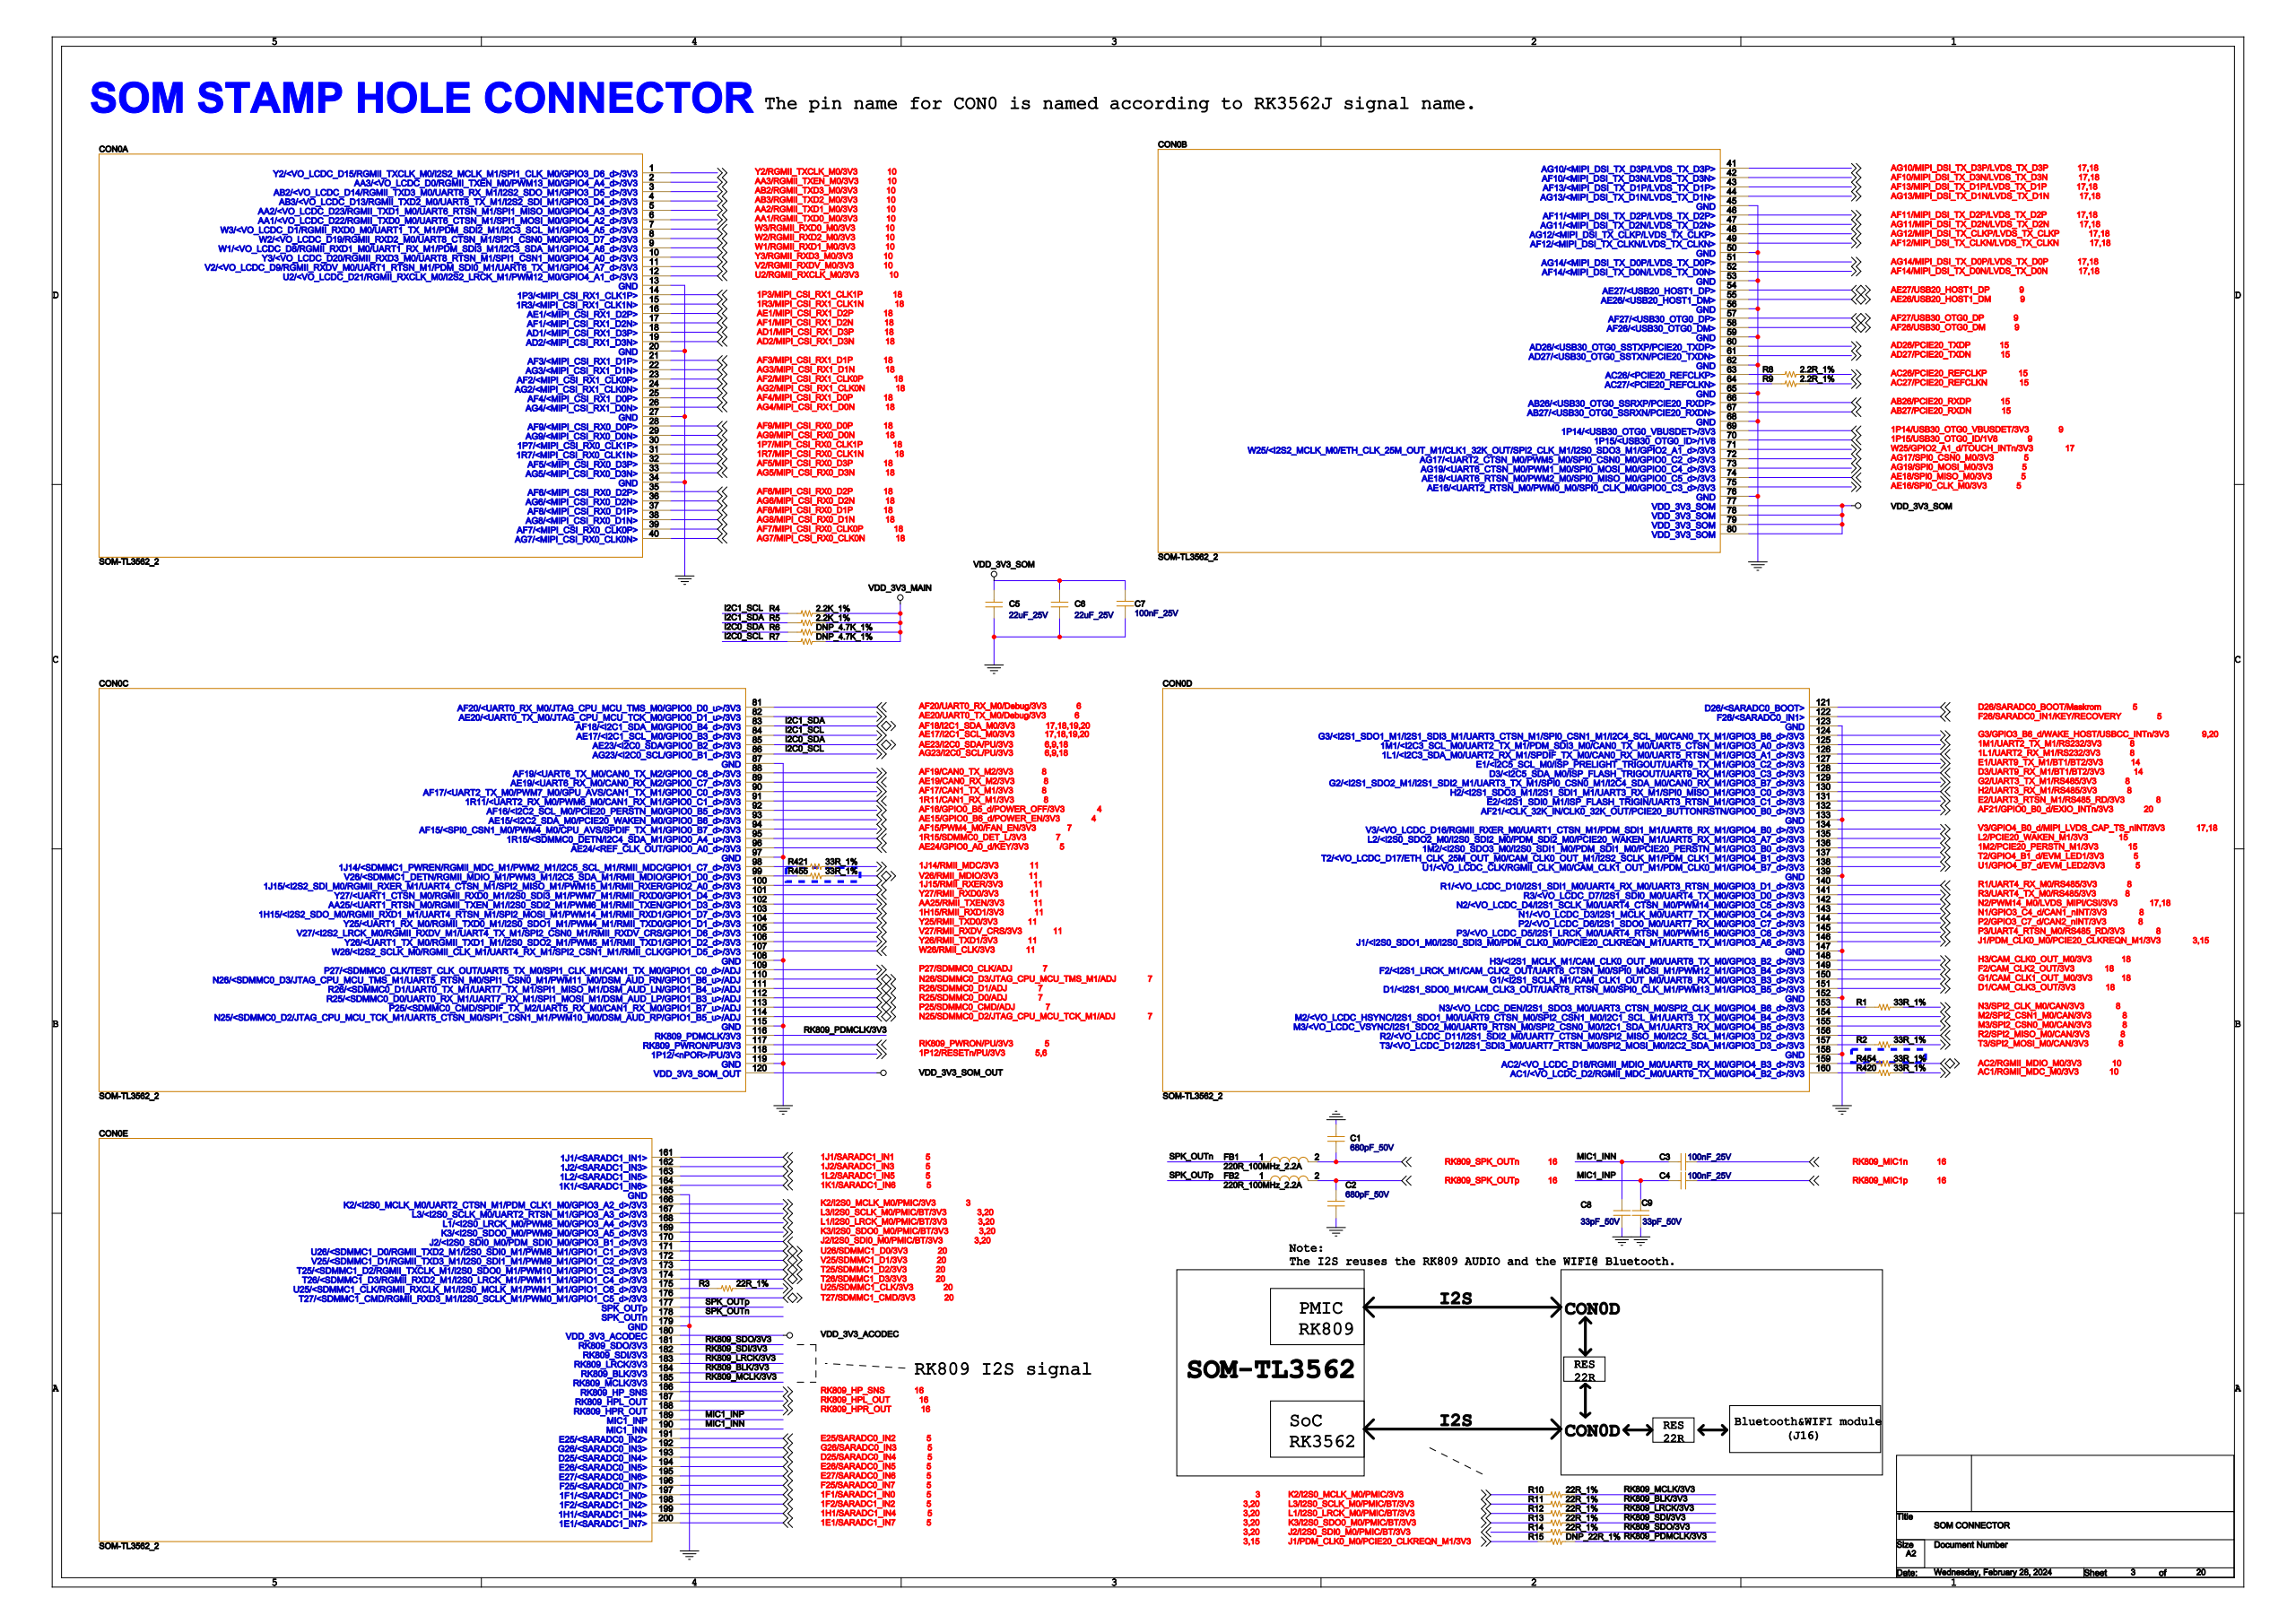Circuit board | Cadence Allegro | 1024 parts | 682 nets | one sheet of the schematic
Parts on this sheet (reference | value | footprint):
C1 | 680pF_50V | C0603
C2 | 680pF_50V | C0603
C3 | 100nF_25V | C0402
C4 | 100nF_25V | C0402
C5 | 22uF_25V | C0805
C6 | 22uF_25V | C0805
C7 | 100nF_25V | C0402
C8 | 33pF_50V | C0603
C9 | 33pF_50V | C0603
CON0 | SMD_200PIN_TL3562 | SMD_200P_45X45_TL3562
FB1 | 220R_100MHz_2A | L0603
FB2 | 220R_100MHz_2A | L0603
R1 | 33R_1% | R0402
R2 | 33R_1% | R0402
R3 | 22R_1% | R0402
R4 | 2.2K_1% | R0603
R5 | 2.2K_1% | R0603
R6 | DNP_4.7K_1% | R0402
R7 | DNP_4.7K_1% | R0402
R8 | 2.2R_1% | R0402
R9 | 2.2R_1% | R0402
R10 | 22R_1% | R0402
R11 | 22R_1% | R0402
R12 | 22R_1% | R0402
R13 | 22R_1% | R0402
R14 | 22R_1% | R0402
R15 | DNP_22R_1% | R0402
R420 | 33R_1% | R0402
R421 | 33R_1% | R0402
R454 | 33R_1% | R0402
R455 | 33R_1% | R0402
Nets of these parts (net: part-pin ...):
GND: C1-2 C2-2 C5-1 C6-1 C7-2 C8-2 C9-2 CON0-13 CON0-20 CON0-27 CON0-34 CON0-45 CON0-50 CON0-53 CON0-56 CON0-59 CON0-62 CON0-65 CON0-68 CON0-76 CON0-87 CON0-97 CON0-108 CON0-115 CON0-119 CON0-123 CON0-133 CON0-139 CON0-147 CON0-152 CON0-158 CON0-165 CON0-179
AG7/MIPI_CSI_RX0_CLK0N: CON0-40
AF7/MIPI_CSI_RX0_CLK0P: CON0-39
1R7/MIPI_CSI_RX0_CLK1N: CON0-31
1P7/MIPI_CSI_RX0_CLK1P: CON0-30
AG9/MIPI_CSI_RX0_D0N: CON0-29
AF9/MIPI_CSI_RX0_D0P: CON0-28
AG8/MIPI_CSI_RX0_D1N: CON0-38
AF8/MIPI_CSI_RX0_D1P: CON0-37
AG6/MIPI_CSI_RX0_D2N: CON0-36
AF6/MIPI_CSI_RX0_D2P: CON0-35
AG5/MIPI_CSI_RX0_D3N: CON0-33
AF5/MIPI_CSI_RX0_D3P: CON0-32
AG2/MIPI_CSI_RX1_CLK0N: CON0-24
AF2/MIPI_CSI_RX1_CLK0P: CON0-23
1R3/MIPI_CSI_RX1_CLK1N: CON0-15
1P3/MIPI_CSI_RX1_CLK1P: CON0-14
AG4/MIPI_CSI_RX1_D0N: CON0-26
AF4/MIPI_CSI_RX1_D0P: CON0-25
AG3/MIPI_CSI_RX1_D1N: CON0-22
AF3/MIPI_CSI_RX1_D1P: CON0-21
AF1/MIPI_CSI_RX1_D2N: CON0-17
AE1/MIPI_CSI_RX1_D2P: CON0-16
AD2/MIPI_CSI_RX1_D3N: CON0-19
AD1/MIPI_CSI_RX1_D3P: CON0-18
VDD_3V3_ACODEC: CON0-180
E25/SARADC0_IN2: CON0-191
1H1/SARADC1_IN4: CON0-199
E27/SARADC0_IN6: CON0-195
1L2/SARADC1_IN5: CON0-163
F25/SARADC0_IN7: CON0-196
1K1/SARADC1_IN6: CON0-164
1E1/SARADC1_IN7: CON0-200
1F1/SARADC1_IN0: CON0-197
1J1/SARADC1_IN1: CON0-161
G26/SARADC0_IN3: CON0-192
1F2/SARADC1_IN2: CON0-198
D25/SARADC0_IN4: CON0-193
1J2/SARADC1_IN3: CON0-162
E26/SARADC0_IN5: CON0-194
VDD_3V3_MAIN: R4-2 R5-2 R6-2 R7-2
1P15/USB30_OTG0_ID/1V8: CON0-70
Y2/RGMII_TXCLK_M0/3V3: CON0-1
Y3/RGMII_RXD3_M0/3V3: CON0-10
V2/RGMII_RXDV_M0/3V3: CON0-11
U2/RGMII_RXCLK_M0/3V3: CON0-12
AA3/RGMII_TXEN_M0/3V3: CON0-2
AB2/RGMII_TXD3_M0/3V3: CON0-3
AB3/RGMII_TXD2_M0/3V3: CON0-4
AA2/RGMII_TXD1_M0/3V3: CON0-5
AA1/RGMII_TXD0_M0/3V3: CON0-6
W3/RGMII_RXD0_M0/3V3: CON0-7
W2/RGMII_RXD2_M0/3V3: CON0-8
W1/RGMII_RXD1_M0/3V3: CON0-9
1J15/RMII_RXER/3V3: CON0-100
AE27/USB20_HOST1_DP: CON0-54
AE26/USB20_HOST1_DM: CON0-55
AF27/USB30_OTG0_DP: CON0-57
AF26/USB30_OTG0_DM: CON0-58
AD26/PCIE20_TXDP: CON0-60
AD27/PCIE20_TXDN: CON0-61
N22276430: R8-1 CON0-63
N22276433: R9-1 CON0-64
AB26/PCIE20_RXDP: CON0-66
AB27/PCIE20_RXDN: CON0-67
1P14/USB30_OTG0_VBUSDET/3V3: CON0-69
AG17/SPI0_CSN0_M0/3V3: CON0-72
AG19/SPI0_MOSI_M0/3V3: CON0-73
AE18/SPI0_MISO_M0/3V3: CON0-74
AE16/SPI0_CLK_M0/3V3: CON0-75
VDD_3V3_SOM: C5-2 C6-2 C7-1 CON0-77 CON0-78 CON0-79 CON0-80
AF18/I2C1_SDA_M0/3V3: R5-1 CON0-83
AE17/I2C1_SCL_M0/3V3: R4-1 CON0-84
AE23/I2C0_SDA/PU/3V3: R6-1 CON0-85
AG23/I2C0_SCL/PU/3V3: R7-1 CON0-86
AF19/CAN0_TX_M2/3V3: CON0-88
AE19/CAN0_RX_M2/3V3: CON0-89
AF17/CAN1_TX_M1/3V3: CON0-90
1R11/CAN1_RX_M1/3V3: CON0-91
AF15/PWM4_M0/FAN_EN/3V3: CON0-94
1R15/SDMMC0_DET_L/3V3: CON0-95
N22276444: R421-1 CON0-98
N22273250: R455-1 CON0-99
Y27/RMII_RXD0/3V3: CON0-101
AA25/RMII_TXEN/3V3: CON0-102
1H15/RMII_RXD1/3V3: CON0-103
Y25/RMII_TXD0/3V3: CON0-104
V27/RMII_RXDV_CRS/3V3: CON0-105
Y26/RMII_TXD1/3V3: CON0-106
W26/RMII_CLK/3V3: CON0-107
P27/SDMMC0_CLK/ADJ: CON0-109
R26/SDMMC0_D1/ADJ: CON0-111
R25/SDMMC0_D0/ADJ: CON0-112
P25/SDMMC0_CMD/ADJ: CON0-113
RK809_PDMCLK/3V3: R15-2 CON0-116
RK809_PWRON/PU/3V3: CON0-117
VDD_3V3_SOM_OUT: CON0-120
F26/SARADC0_IN1/KEY/RECOVERY: CON0-122
1M1/UART2_TX_M1/RS232/3V3: CON0-125
1L1/UART2_RX_M1/RS232/3V3: CON0-126
E1/UART9_TX_M1/BT1/BT2/3V3: CON0-127
D3/UART9_RX_M1/BT1/BT2/3V3: CON0-128
G2/UART3_TX_M1/RS485/3V3: CON0-129
H2/UART3_RX_M1/RS485/3V3: CON0-130
E2/UART3_RTSN_M1/RS485_RD/3V3: CON0-131
L2/PCIE20_WAKEN_M1/3V3: CON0-135
1M2/PCIE20_PERSTN_M1/3V3: CON0-136
R1/UART4_RX_M0/RS485/3V3: CON0-140
R3/UART4_TX_M0/RS485/3V3: CON0-141
N2/PWM14_M0/LVDS_MIPI/CSI/3V3: CON0-142
P3/UART4_RTSN_M0/RS485_RD/3V3: CON0-145
J1/PDM_CLK0_M0/PCIE20_CLKREQN_M: R15-1 CON0-146
H3/CAM_CLK0_OUT_M0/3V3: CON0-148
F2/CAM_CLK2_OUT/3V3: CON0-149
G1/CAM_CLK1_OUT_M0/3V3: CON0-150
D1/CAM_CLK3_OUT/3V3: CON0-151
N22280460: R1-1 CON0-153
M2/SPI2_CSN1_M0/CAN/3V3: CON0-154
M3/SPI2_CSN0_M0/CAN/3V3: CON0-155
R2/SPI2_MISO_M0/CAN/3V3: CON0-156
N22280440: R2-1 CON0-157
N22221258: R454-1 CON0-159
N22232910: R420-1 CON0-160
K2/I2S0_MCLK_M0/PMIC/3V3: R10-1 CON0-166
L3/I2S0_SCLK_M0/PMIC/BT/3V3: R11-1 CON0-167
L1/I2S0_LRCK_M0/PMIC/BT/3V3: R12-1 CON0-168
K3/I2S0_SDO0_M0/PMIC/BT/3V3: R13-1 CON0-169
J2/I2S0_SDI0_M0/PMIC/BT/3V3: R14-1 CON0-170
U26/SDMMC1_D0/3V3: CON0-171
V25/SDMMC1_D1/3V3: CON0-172
T25/SDMMC1_D2/3V3: CON0-173
T26/SDMMC1_D3/3V3: CON0-174
N22232897: R3-1 CON0-175
T27/SDMMC1_CMD/3V3: CON0-176
SPK_OUTP: FB2-1 CON0-177
SPK_OUTN: FB1-1 CON0-178
RK809_SDO/3V3: R14-2 CON0-181
RK809_SDI/3V3: R13-2 CON0-182
RK809_LRCK/3V3: R12-2 CON0-183
RK809_BLK/3V3: R11-2 CON0-184
RK809_MCLK/3V3: R10-2 CON0-185
RK809_HP_SNS: CON0-186
RK809_HPL_OUT: CON0-187
RK809_HPR_OUT: CON0-188
MIC1_INP: C4-2 C9-1 CON0-189
MIC1_INN: C3-2 C8-1 CON0-190
AC2/RGMII_MDIO_M0/3V3: R454-2
V26/RMII_MDIO/3V3: R455-2
N3/SPI2_CLK_M0/CAN/3V3: R1-2
T3/SPI2_MOSI_M0/CAN/3V3: R2-2
1J14/RMII_MDC/3V3: R421-2
RK809_SPK_OUTP: C2-1 FB2-2
RK809_SPK_OUTN: C1-1 FB1-2
RK809_MIC1P: C4-1
RK809_MIC1N: C3-1
U25/SDMMC1_CLK/3V3: R3-2
AC26/PCIE20_REFCLKP: R8-2
AC27/PCIE20_REFCLKN: R9-2
AC1/RGMII_MDC_M0/3V3: R420-2